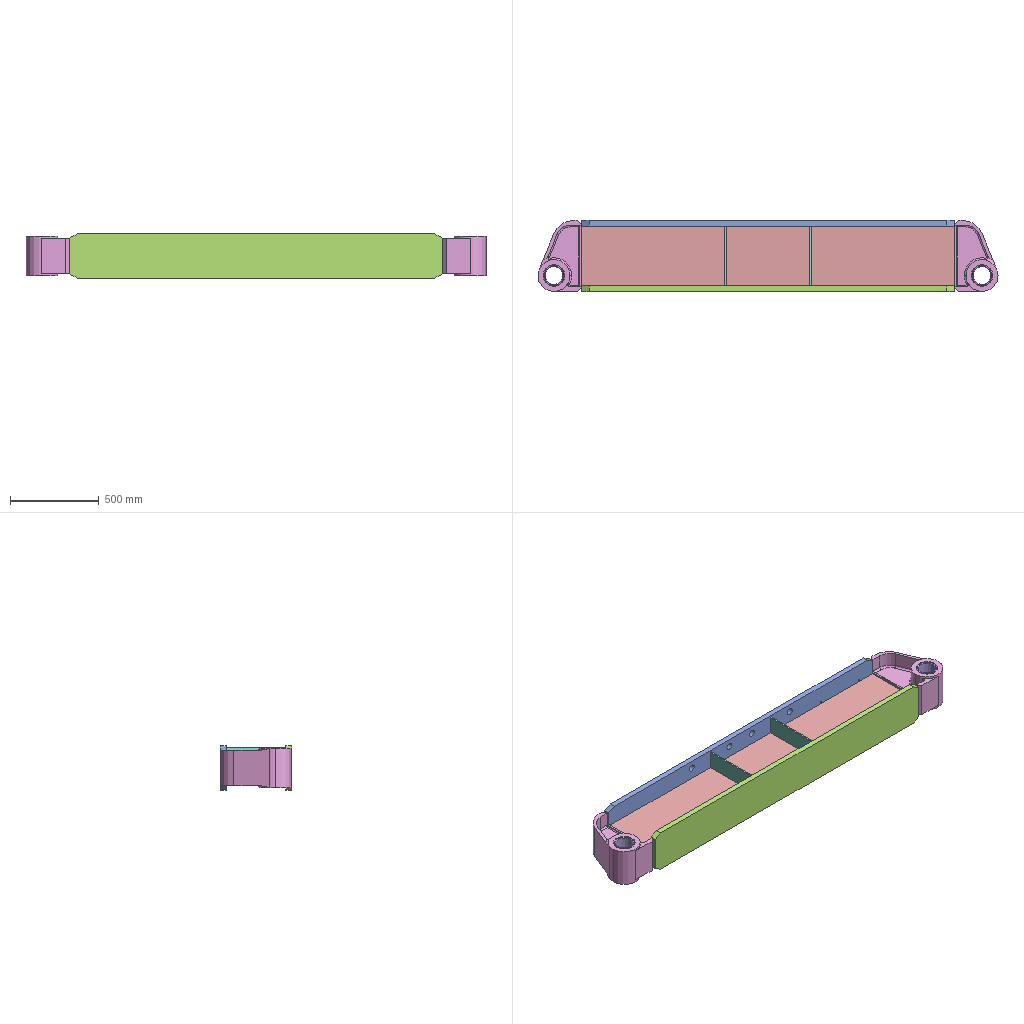Assembly | SolidWorks | 7 different items | 13 placed | box 2590 x 400 x 250 mm
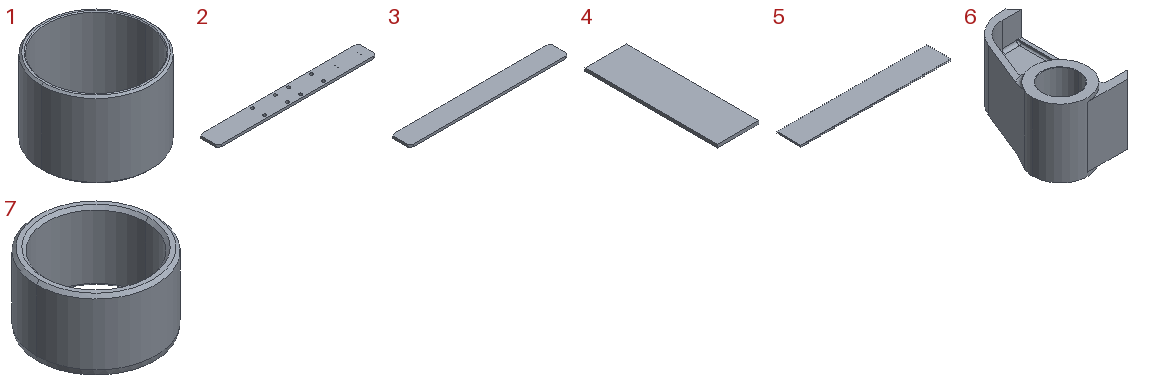Parts list (item | quantity | size | volume | features):
1 | x2 | 120 x 120 x 84 mm | 149900 mm3 | features Chamfer 2, Extrusion 1
2 | x1 | 2100 x 250 x 32 mm | 16420254 mm3 | features Extrusion 1, HoleWzd 1, LPattern 1
3 | x1 | 2100 x 250 x 32 mm | 16730718 mm3 | features Extrusion 1
4 | x2 | 105 x 336 x 8 mm | 282240 mm3 | features Extrusion 1
5 | x1 | 2100 x 336 x 20 mm | 14112000 mm3 | features Extrusion 1
6 | x2 | 245 x 400 x 225 mm | 5993889 mm3 | features Fillet 4, ICE 4, Chamfer 2, Extrusion 1
7 | x4 | 120 x 120 x 70 mm | 236524 mm3 | features Chamfer 2, Extrusion 1
Mates (type | each side: item.copy, entity, surface, feature):
Coincident | 1.1 plane | assembly plane
Parallel | 1.1 plane | assembly plane
Coincident | 1.2 plane | assembly plane
Parallel | 1.2 plane | assembly plane
Coincident | 1.2 face plane Boss-Extrude1 | 7.1 face plane Boss-Extrude1
Parallel | 7.1 plane | assembly plane
Coincident | 5.1 face plane Boss-Extrude1 | 2.1 face plane Boss-Extrude1
Coincident | 5.1 face plane Boss-Extrude1 | 3.1 face plane Boss-Extrude1
Coincident | 5.1 face plane Boss-Extrude1 | 4.1 face plane Boss-Extrude1
Coincident | 2.1 face plane Boss-Extrude1 | 6.1 face plane Boss-Extrude1 | 2 times
Coincident | 2.1 face plane Boss-Extrude1 | 6.2 face plane Boss-Extrude1 | 2 times
Coincident | 2.1 face plane Boss-Extrude1 | 4.1 face plane Boss-Extrude1
Concentric | 6.1 face cylinder Cut-Extrude1 | 1.1 face cylinder Boss-Extrude1
Concentric | 6.2 face cylinder Cut-Extrude1 | 1.2 face cylinder Boss-Extrude1
Concentric | 6.2 face cylinder Cut-Extrude1 | 7.1 face cylinder Boss-Extrude1